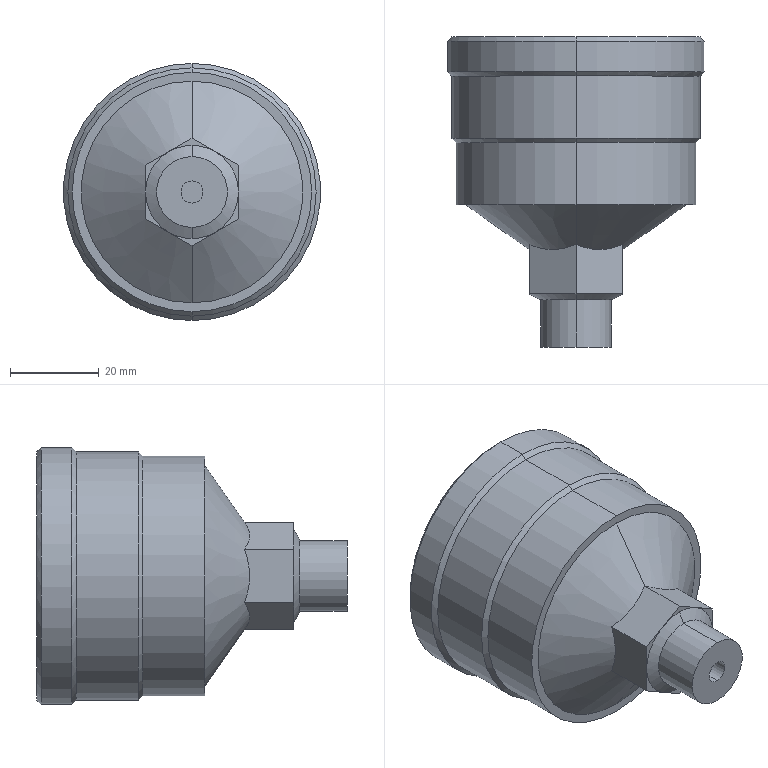Part | SolidWorks | features Boss 1, Revolution 1 | 1 solid | 41 faces | box 58 x 70 x 58 mm | volume 93422 mm3 | plane 17 | cylinder 12 | cone 12 | commonest cylinder face diameters 5 x2 16 x2 26.006 x2 54 x2 56 x2 58 x2
STEP:
#1=CARTESIAN_POINT('',(0.,0.,-2.5));
#2=VERTEX_POINT('',#1);
#3=CARTESIAN_POINT('',(0.,0.,2.5));
#4=VERTEX_POINT('',#3);
#5=CARTESIAN_POINT('',(0.,0.,0.));
#6=DIRECTION('',(0.,1.,0.));
#7=DIRECTION('',(0.,0.,1.));
#8=AXIS2_PLACEMENT_3D('',#5,#6,#7);
#9=CIRCLE('',#8,2.5);
#10=EDGE_CURVE('',#2,#4,#9,.T.);
#11=ORIENTED_EDGE('',*,*,#10,.F.);
#12=CARTESIAN_POINT('',(0.,12.,-2.5));
#13=VERTEX_POINT('',#12);
#14=CARTESIAN_POINT('',(0.,0.,-2.5));
#15=DIRECTION('',(0.,1.,0.));
#16=VECTOR('',#15,1000.);
#17=LINE('',#14,#16);
#18=EDGE_CURVE('',#2,#13,#17,.T.);
#19=ORIENTED_EDGE('',*,*,#18,.T.);
#20=CARTESIAN_POINT('',(0.,12.,2.5));
#21=VERTEX_POINT('',#20);
#22=CARTESIAN_POINT('',(0.,12.,0.));
#23=DIRECTION('',(0.,-1.,0.));
#24=DIRECTION('',(0.,0.,-1.));
#25=AXIS2_PLACEMENT_3D('',#22,#23,#24);
#26=CIRCLE('',#25,2.5);
#27=EDGE_CURVE('',#21,#13,#26,.T.);
#28=ORIENTED_EDGE('',*,*,#27,.F.);
#29=CARTESIAN_POINT('',(0.,0.,2.5));
#30=DIRECTION('',(0.,1.,0.));
#31=VECTOR('',#30,1000.);
#32=LINE('',#29,#31);
#33=EDGE_CURVE('',#4,#21,#32,.T.);
#34=ORIENTED_EDGE('',*,*,#33,.F.);
#35=EDGE_LOOP('',(#11,#19,#28,#34));
#36=FACE_OUTER_BOUND('',#35,.T.);
#37=CARTESIAN_POINT('',(0.,0.,0.));
#38=DIRECTION('',(0.,1.,0.));
#39=DIRECTION('',(0.,0.,1.));
#40=AXIS2_PLACEMENT_3D('',#37,#38,#39);
#41=CYLINDRICAL_SURFACE('',#40,2.5);
#42=ADVANCED_FACE('',(#36),#41,.F.);
#43=CARTESIAN_POINT('',(0.,10.699,8.));
#44=VERTEX_POINT('',#43);
#45=CARTESIAN_POINT('',(0.,10.699,-8.));
#46=VERTEX_POINT('',#45);
#47=CARTESIAN_POINT('',(0.,10.699,0.));
#48=DIRECTION('',(0.,1.,0.));
#49=DIRECTION('',(0.,0.,1.));
#50=AXIS2_PLACEMENT_3D('',#47,#48,#49);
#51=CIRCLE('',#50,8.);
#52=EDGE_CURVE('',#44,#46,#51,.T.);
#53=ORIENTED_EDGE('',*,*,#52,.T.);
#54=CARTESIAN_POINT('',(0.,12.,-10.5));
#55=VERTEX_POINT('',#54);
#56=CARTESIAN_POINT('',(0.,12.,-10.5));
#57=DIRECTION('',(0.,0.4617,-0.887));
#58=VECTOR('',#57,1000.);
#59=LINE('',#56,#58);
#60=EDGE_CURVE('',#46,#55,#59,.T.);
#61=ORIENTED_EDGE('',*,*,#60,.T.);
#62=CARTESIAN_POINT('',(5.25,12.,-9.093));
#63=VERTEX_POINT('',#62);
#64=CARTESIAN_POINT('',(0.,12.,0.));
#65=DIRECTION('',(0.,1.,0.));
#66=DIRECTION('',(0.,0.,1.));
#67=AXIS2_PLACEMENT_3D('',#64,#65,#66);
#68=CIRCLE('',#67,10.5);
#69=EDGE_CURVE('',#63,#55,#68,.T.);
#70=ORIENTED_EDGE('',*,*,#69,.F.);
#71=CARTESIAN_POINT('',(10.5,12.,0.));
#72=VERTEX_POINT('',#71);
#73=CARTESIAN_POINT('',(0.,12.,0.));
#74=DIRECTION('',(0.,1.,0.));
#75=DIRECTION('',(0.,0.,1.));
#76=AXIS2_PLACEMENT_3D('',#73,#74,#75);
#77=CIRCLE('',#76,10.5);
#78=EDGE_CURVE('',#72,#63,#77,.T.);
#79=ORIENTED_EDGE('',*,*,#78,.F.);
#80=CARTESIAN_POINT('',(5.25,12.,9.093));
#81=VERTEX_POINT('',#80);
#82=CARTESIAN_POINT('',(0.,12.,0.));
#83=DIRECTION('',(0.,1.,0.));
#84=DIRECTION('',(0.,0.,1.));
#85=AXIS2_PLACEMENT_3D('',#82,#83,#84);
#86=CIRCLE('',#85,10.5);
#87=EDGE_CURVE('',#81,#72,#86,.T.);
#88=ORIENTED_EDGE('',*,*,#87,.F.);
#89=CARTESIAN_POINT('',(0.,12.,10.5));
#90=VERTEX_POINT('',#89);
#91=CARTESIAN_POINT('',(0.,12.,0.));
#92=DIRECTION('',(0.,1.,0.));
#93=DIRECTION('',(0.,0.,1.));
#94=AXIS2_PLACEMENT_3D('',#91,#92,#93);
#95=CIRCLE('',#94,10.5);
#96=EDGE_CURVE('',#90,#81,#95,.T.);
#97=ORIENTED_EDGE('',*,*,#96,.F.);
#98=CARTESIAN_POINT('',(0.,12.,10.5));
#99=DIRECTION('',(0.,0.4617,0.887));
#100=VECTOR('',#99,1000.);
#101=LINE('',#98,#100);
#102=EDGE_CURVE('',#44,#90,#101,.T.);
#103=ORIENTED_EDGE('',*,*,#102,.F.);
#104=EDGE_LOOP('',(#53,#61,#70,#79,#88,#97,#103));
#105=FACE_OUTER_BOUND('',#104,.T.);
#106=CARTESIAN_POINT('',(0.,12.,0.));
#107=DIRECTION('',(0.,1.,0.));
#108=DIRECTION('',(0.,0.,1.));
#109=AXIS2_PLACEMENT_3D('',#106,#107,#108);
#110=CONICAL_SURFACE('',#109,10.5,1.091);
#111=ADVANCED_FACE('',(#105),#110,.T.);
#112=CARTESIAN_POINT('',(0.,0.,8.));
#113=VERTEX_POINT('',#112);
#114=CARTESIAN_POINT('',(0.,0.,-8.));
#115=VERTEX_POINT('',#114);
#116=CARTESIAN_POINT('',(0.,0.,0.));
#117=DIRECTION('',(0.,1.,0.));
#118=DIRECTION('',(0.,0.,1.));
#119=AXIS2_PLACEMENT_3D('',#116,#117,#118);
#120=CIRCLE('',#119,8.);
#121=EDGE_CURVE('',#113,#115,#120,.T.);
#122=ORIENTED_EDGE('',*,*,#121,.T.);
#123=CARTESIAN_POINT('',(0.,0.,-8.));
#124=DIRECTION('',(0.,1.,0.));
#125=VECTOR('',#124,1000.);
#126=LINE('',#123,#125);
#127=EDGE_CURVE('',#115,#46,#126,.T.);
#128=ORIENTED_EDGE('',*,*,#127,.T.);
#129=ORIENTED_EDGE('',*,*,#52,.F.);
#130=CARTESIAN_POINT('',(0.,0.,8.));
#131=DIRECTION('',(0.,1.,0.));
#132=VECTOR('',#131,1000.);
#133=LINE('',#130,#132);
#134=EDGE_CURVE('',#113,#44,#133,.T.);
#135=ORIENTED_EDGE('',*,*,#134,.F.);
#136=EDGE_LOOP('',(#122,#128,#129,#135));
#137=FACE_OUTER_BOUND('',#136,.T.);
#138=CARTESIAN_POINT('',(0.,0.,0.));
#139=DIRECTION('',(0.,1.,0.));
#140=DIRECTION('',(0.,0.,1.));
#141=AXIS2_PLACEMENT_3D('',#138,#139,#140);
#142=CYLINDRICAL_SURFACE('',#141,8.);
#143=ADVANCED_FACE('',(#137),#142,.T.);
#144=CARTESIAN_POINT('',(0.,70.,28.));
#145=VERTEX_POINT('',#144);
#146=CARTESIAN_POINT('',(0.,70.,-28.));
#147=VERTEX_POINT('',#146);
#148=CARTESIAN_POINT('',(0.,70.,0.));
#149=DIRECTION('',(0.,1.,0.));
#150=DIRECTION('',(0.,0.,1.));
#151=AXIS2_PLACEMENT_3D('',#148,#149,#150);
#152=CIRCLE('',#151,28.);
#153=EDGE_CURVE('',#145,#147,#152,.T.);
#154=ORIENTED_EDGE('',*,*,#153,.F.);
#155=CARTESIAN_POINT('',(0.,69.,29.));
#156=VERTEX_POINT('',#155);
#157=CARTESIAN_POINT('',(0.,70.,28.));
#158=DIRECTION('',(0.,-0.7071,0.7071));
#159=VECTOR('',#158,1000.);
#160=LINE('',#157,#159);
#161=EDGE_CURVE('',#145,#156,#160,.T.);
#162=ORIENTED_EDGE('',*,*,#161,.T.);
#163=CARTESIAN_POINT('',(0.,69.,-29.));
#164=VERTEX_POINT('',#163);
#165=CARTESIAN_POINT('',(0.,69.,0.));
#166=DIRECTION('',(0.,1.,0.));
#167=DIRECTION('',(0.,0.,1.));
#168=AXIS2_PLACEMENT_3D('',#165,#166,#167);
#169=CIRCLE('',#168,29.);
#170=EDGE_CURVE('',#156,#164,#169,.T.);
#171=ORIENTED_EDGE('',*,*,#170,.T.);
#172=CARTESIAN_POINT('',(0.,70.,-28.));
#173=DIRECTION('',(0.,-0.7071,-0.7071));
#174=VECTOR('',#173,1000.);
#175=LINE('',#172,#174);
#176=EDGE_CURVE('',#147,#164,#175,.T.);
#177=ORIENTED_EDGE('',*,*,#176,.F.);
#178=EDGE_LOOP('',(#154,#162,#171,#177));
#179=FACE_OUTER_BOUND('',#178,.T.);
#180=CARTESIAN_POINT('',(0.,70.,0.));
#181=DIRECTION('',(0.,-1.,0.));
#182=DIRECTION('',(0.,0.,-1.));
#183=AXIS2_PLACEMENT_3D('',#180,#181,#182);
#184=CONICAL_SURFACE('',#183,28.,0.7854);
#185=ADVANCED_FACE('',(#179),#184,.T.);
#186=CARTESIAN_POINT('',(0.,62.153,29.));
#187=VERTEX_POINT('',#186);
#188=CARTESIAN_POINT('',(0.,62.153,-29.));
#189=VERTEX_POINT('',#188);
#190=CARTESIAN_POINT('',(0.,62.153,0.));
#191=DIRECTION('',(0.,1.,0.));
#192=DIRECTION('',(0.,0.,1.));
#193=AXIS2_PLACEMENT_3D('',#190,#191,#192);
#194=CIRCLE('',#193,29.);
#195=EDGE_CURVE('',#187,#189,#194,.T.);
#196=ORIENTED_EDGE('',*,*,#195,.T.);
#197=CARTESIAN_POINT('',(0.,0.,-29.));
#198=DIRECTION('',(0.,1.,0.));
#199=VECTOR('',#198,1000.);
#200=LINE('',#197,#199);
#201=EDGE_CURVE('',#189,#164,#200,.T.);
#202=ORIENTED_EDGE('',*,*,#201,.T.);
#203=ORIENTED_EDGE('',*,*,#170,.F.);
#204=CARTESIAN_POINT('',(0.,0.,29.));
#205=DIRECTION('',(0.,1.,0.));
#206=VECTOR('',#205,1000.);
#207=LINE('',#204,#206);
#208=EDGE_CURVE('',#187,#156,#207,.T.);
#209=ORIENTED_EDGE('',*,*,#208,.F.);
#210=EDGE_LOOP('',(#196,#202,#203,#209));
#211=FACE_OUTER_BOUND('',#210,.T.);
#212=CARTESIAN_POINT('',(0.,0.,0.));
#213=DIRECTION('',(0.,1.,0.));
#214=DIRECTION('',(0.,0.,1.));
#215=AXIS2_PLACEMENT_3D('',#212,#213,#214);
#216=CYLINDRICAL_SURFACE('',#215,29.);
#217=ADVANCED_FACE('',(#211),#216,.T.);
#218=CARTESIAN_POINT('',(0.,61.153,28.));
#219=VERTEX_POINT('',#218);
#220=CARTESIAN_POINT('',(0.,61.153,-28.));
#221=VERTEX_POINT('',#220);
#222=CARTESIAN_POINT('',(0.,61.153,0.));
#223=DIRECTION('',(0.,1.,0.));
#224=DIRECTION('',(0.,0.,1.));
#225=AXIS2_PLACEMENT_3D('',#222,#223,#224);
#226=CIRCLE('',#225,28.);
#227=EDGE_CURVE('',#219,#221,#226,.T.);
#228=ORIENTED_EDGE('',*,*,#227,.T.);
#229=CARTESIAN_POINT('',(0.,62.153,-29.));
#230=DIRECTION('',(0.,0.7071,-0.7071));
#231=VECTOR('',#230,1000.);
#232=LINE('',#229,#231);
#233=EDGE_CURVE('',#221,#189,#232,.T.);
#234=ORIENTED_EDGE('',*,*,#233,.T.);
#235=ORIENTED_EDGE('',*,*,#195,.F.);
#236=CARTESIAN_POINT('',(0.,62.153,29.));
#237=DIRECTION('',(0.,0.7071,0.7071));
#238=VECTOR('',#237,1000.);
#239=LINE('',#236,#238);
#240=EDGE_CURVE('',#219,#187,#239,.T.);
#241=ORIENTED_EDGE('',*,*,#240,.F.);
#242=EDGE_LOOP('',(#228,#234,#235,#241));
#243=FACE_OUTER_BOUND('',#242,.T.);
#244=CARTESIAN_POINT('',(0.,62.153,0.));
#245=DIRECTION('',(0.,1.,0.));
#246=DIRECTION('',(0.,0.,1.));
#247=AXIS2_PLACEMENT_3D('',#244,#245,#246);
#248=CONICAL_SURFACE('',#247,29.,0.7854);
#249=ADVANCED_FACE('',(#243),#248,.T.);
#250=CARTESIAN_POINT('',(0.,47.153,28.));
#251=VERTEX_POINT('',#250);
#252=CARTESIAN_POINT('',(0.,47.153,-28.));
#253=VERTEX_POINT('',#252);
#254=CARTESIAN_POINT('',(0.,47.153,0.));
#255=DIRECTION('',(0.,1.,0.));
#256=DIRECTION('',(0.,0.,1.));
#257=AXIS2_PLACEMENT_3D('',#254,#255,#256);
#258=CIRCLE('',#257,28.);
#259=EDGE_CURVE('',#251,#253,#258,.T.);
#260=ORIENTED_EDGE('',*,*,#259,.T.);
#261=CARTESIAN_POINT('',(0.,0.,-28.));
#262=DIRECTION('',(0.,1.,0.));
#263=VECTOR('',#262,1000.);
#264=LINE('',#261,#263);
#265=EDGE_CURVE('',#253,#221,#264,.T.);
#266=ORIENTED_EDGE('',*,*,#265,.T.);
#267=ORIENTED_EDGE('',*,*,#227,.F.);
#268=CARTESIAN_POINT('',(0.,0.,28.));
#269=DIRECTION('',(0.,1.,0.));
#270=VECTOR('',#269,1000.);
#271=LINE('',#268,#270);
#272=EDGE_CURVE('',#251,#219,#271,.T.);
#273=ORIENTED_EDGE('',*,*,#272,.F.);
#274=EDGE_LOOP('',(#260,#266,#267,#273));
#275=FACE_OUTER_BOUND('',#274,.T.);
#276=CARTESIAN_POINT('',(0.,0.,0.));
#277=DIRECTION('',(0.,1.,0.));
#278=DIRECTION('',(0.,0.,1.));
#279=AXIS2_PLACEMENT_3D('',#276,#277,#278);
#280=CYLINDRICAL_SURFACE('',#279,28.);
#281=ADVANCED_FACE('',(#275),#280,.T.);
#282=CARTESIAN_POINT('',(0.,46.153,27.));
#283=VERTEX_POINT('',#282);
#284=CARTESIAN_POINT('',(0.,46.153,-27.));
#285=VERTEX_POINT('',#284);
#286=CARTESIAN_POINT('',(0.,46.153,0.));
#287=DIRECTION('',(0.,1.,0.));
#288=DIRECTION('',(0.,0.,1.));
#289=AXIS2_PLACEMENT_3D('',#286,#287,#288);
#290=CIRCLE('',#289,27.);
#291=EDGE_CURVE('',#283,#285,#290,.T.);
#292=ORIENTED_EDGE('',*,*,#291,.T.);
#293=CARTESIAN_POINT('',(0.,47.153,-28.));
#294=DIRECTION('',(0.,0.7071,-0.7071));
#295=VECTOR('',#294,1000.);
#296=LINE('',#293,#295);
#297=EDGE_CURVE('',#285,#253,#296,.T.);
#298=ORIENTED_EDGE('',*,*,#297,.T.);
#299=ORIENTED_EDGE('',*,*,#259,.F.);
#300=CARTESIAN_POINT('',(0.,47.153,28.));
#301=DIRECTION('',(0.,0.7071,0.7071));
#302=VECTOR('',#301,1000.);
#303=LINE('',#300,#302);
#304=EDGE_CURVE('',#283,#251,#303,.T.);
#305=ORIENTED_EDGE('',*,*,#304,.F.);
#306=EDGE_LOOP('',(#292,#298,#299,#305));
#307=FACE_OUTER_BOUND('',#306,.T.);
#308=CARTESIAN_POINT('',(0.,47.153,0.));
#309=DIRECTION('',(0.,1.,0.));
#310=DIRECTION('',(0.,0.,1.));
#311=AXIS2_PLACEMENT_3D('',#308,#309,#310);
#312=CONICAL_SURFACE('',#311,28.,0.7854);
#313=ADVANCED_FACE('',(#307),#312,.T.);
#314=CARTESIAN_POINT('',(0.,32.153,27.));
#315=VERTEX_POINT('',#314);
#316=CARTESIAN_POINT('',(0.,32.153,-27.));
#317=VERTEX_POINT('',#316);
#318=CARTESIAN_POINT('',(0.,32.153,0.));
#319=DIRECTION('',(0.,1.,0.));
#320=DIRECTION('',(0.,0.,1.));
#321=AXIS2_PLACEMENT_3D('',#318,#319,#320);
#322=CIRCLE('',#321,27.);
#323=EDGE_CURVE('',#315,#317,#322,.T.);
#324=ORIENTED_EDGE('',*,*,#323,.T.);
#325=CARTESIAN_POINT('',(0.,0.,-27.));
#326=DIRECTION('',(0.,1.,0.));
#327=VECTOR('',#326,1000.);
#328=LINE('',#325,#327);
#329=EDGE_CURVE('',#317,#285,#328,.T.);
#330=ORIENTED_EDGE('',*,*,#329,.T.);
#331=ORIENTED_EDGE('',*,*,#291,.F.);
#332=CARTESIAN_POINT('',(0.,0.,27.));
#333=DIRECTION('',(0.,1.,0.));
#334=VECTOR('',#333,1000.);
#335=LINE('',#332,#334);
#336=EDGE_CURVE('',#315,#283,#335,.T.);
#337=ORIENTED_EDGE('',*,*,#336,.F.);
#338=EDGE_LOOP('',(#324,#330,#331,#337));
#339=FACE_OUTER_BOUND('',#338,.T.);
#340=CARTESIAN_POINT('',(0.,0.,0.));
#341=DIRECTION('',(0.,1.,0.));
#342=DIRECTION('',(0.,0.,1.));
#343=AXIS2_PLACEMENT_3D('',#340,#341,#342);
#344=CYLINDRICAL_SURFACE('',#343,27.);
#345=ADVANCED_FACE('',(#339),#344,.T.);
#346=CARTESIAN_POINT('',(0.,32.153,-2.5));
#347=VERTEX_POINT('',#346);
#348=CARTESIAN_POINT('',(0.,32.153,2.5));
#349=VERTEX_POINT('',#348);
#350=CARTESIAN_POINT('',(0.,32.153,0.));
#351=DIRECTION('',(0.,1.,0.));
#352=DIRECTION('',(0.,0.,1.));
#353=AXIS2_PLACEMENT_3D('',#350,#351,#352);
#354=CIRCLE('',#353,2.5);
#355=EDGE_CURVE('',#347,#349,#354,.T.);
#356=ORIENTED_EDGE('',*,*,#355,.F.);
#357=CARTESIAN_POINT('',(0.,47.153,-13.003));
#358=VERTEX_POINT('',#357);
#359=CARTESIAN_POINT('',(0.,32.153,-2.5));
#360=DIRECTION('',(0.,0.8192,-0.5736));
#361=VECTOR('',#360,1000.);
#362=LINE('',#359,#361);
#363=EDGE_CURVE('',#347,#358,#362,.T.);
#364=ORIENTED_EDGE('',*,*,#363,.T.);
#365=CARTESIAN_POINT('',(0.,47.153,13.003));
#366=VERTEX_POINT('',#365);
#367=CARTESIAN_POINT('',(0.,47.153,0.));
#368=DIRECTION('',(0.,1.,0.));
#369=DIRECTION('',(0.,0.,1.));
#370=AXIS2_PLACEMENT_3D('',#367,#368,#369);
#371=CIRCLE('',#370,13.003);
#372=EDGE_CURVE('',#358,#366,#371,.T.);
#373=ORIENTED_EDGE('',*,*,#372,.T.);
#374=CARTESIAN_POINT('',(0.,32.153,2.5));
#375=DIRECTION('',(0.,0.8192,0.5736));
#376=VECTOR('',#375,1000.);
#377=LINE('',#374,#376);
#378=EDGE_CURVE('',#349,#366,#377,.T.);
#379=ORIENTED_EDGE('',*,*,#378,.F.);
#380=EDGE_LOOP('',(#356,#364,#373,#379));
#381=FACE_OUTER_BOUND('',#380,.T.);
#382=CARTESIAN_POINT('',(0.,32.153,0.));
#383=DIRECTION('',(0.,1.,0.));
#384=DIRECTION('',(0.,0.,1.));
#385=AXIS2_PLACEMENT_3D('',#382,#383,#384);
#386=CONICAL_SURFACE('',#385,2.5,0.6109);
#387=ADVANCED_FACE('',(#381),#386,.F.);
#388=ORIENTED_EDGE('',*,*,#372,.F.);
#389=CARTESIAN_POINT('',(0.,70.,-13.003));
#390=VERTEX_POINT('',#389);
#391=CARTESIAN_POINT('',(0.,0.,-13.003));
#392=DIRECTION('',(0.,1.,0.));
#393=VECTOR('',#392,1000.);
#394=LINE('',#391,#393);
#395=EDGE_CURVE('',#358,#390,#394,.T.);
#396=ORIENTED_EDGE('',*,*,#395,.T.);
#397=CARTESIAN_POINT('',(0.,70.,13.003));
#398=VERTEX_POINT('',#397);
#399=CARTESIAN_POINT('',(0.,70.,0.));
#400=DIRECTION('',(0.,1.,0.));
#401=DIRECTION('',(0.,0.,1.));
#402=AXIS2_PLACEMENT_3D('',#399,#400,#401);
#403=CIRCLE('',#402,13.003);
#404=EDGE_CURVE('',#390,#398,#403,.T.);
#405=ORIENTED_EDGE('',*,*,#404,.T.);
#406=CARTESIAN_POINT('',(0.,0.,13.003));
#407=DIRECTION('',(0.,1.,0.));
#408=VECTOR('',#407,1000.);
#409=LINE('',#406,#408);
#410=EDGE_CURVE('',#366,#398,#409,.T.);
#411=ORIENTED_EDGE('',*,*,#410,.F.);
#412=EDGE_LOOP('',(#388,#396,#405,#411));
#413=FACE_OUTER_BOUND('',#412,.T.);
#414=CARTESIAN_POINT('',(0.,0.,0.));
#415=DIRECTION('',(0.,1.,0.));
#416=DIRECTION('',(0.,0.,1.));
#417=AXIS2_PLACEMENT_3D('',#414,#415,#416);
#418=CYLINDRICAL_SURFACE('',#417,13.003);
#419=ADVANCED_FACE('',(#413),#418,.F.);
#420=CARTESIAN_POINT('',(10.5,23.137,-6.062));
#421=VERTEX_POINT('',#420);
#422=CARTESIAN_POINT('',(0.,23.137,-12.124));
#423=VERTEX_POINT('',#422);
#424=CARTESIAN_POINT('',(10.5,23.137,-6.062));
#425=CARTESIAN_POINT('',(9.651,22.794,-6.552));
#426=CARTESIAN_POINT('',(8.793,22.509,-7.048));
#427=CARTESIAN_POINT('',(7.053,22.113,-8.053));
#428=CARTESIAN_POINT('',(6.17,22.002,-8.562));
#429=CARTESIAN_POINT('',(4.821,21.999,-9.341));
#430=CARTESIAN_POINT('',(4.366,22.026,-9.603));
#431=CARTESIAN_POINT('',(3.472,22.131,-10.12));
#432=CARTESIAN_POINT('',(3.03,22.208,-10.375));
#433=CARTESIAN_POINT('',(1.713,22.507,-11.135));
#434=CARTESIAN_POINT('',(0.8515,22.793,-11.633));
#435=CARTESIAN_POINT('',(0.,23.137,-12.124));
#436=B_SPLINE_CURVE_WITH_KNOTS('',3,(#424,#425,#426,#427,#428,#429,#430,#431,#432,#433,#434,#435),.UNSPECIFIED.,.F.,.F.,(4,2,2,2,2,4),(0.000000241,0.003072,0.006144,0.00768,0.009216,0.01229),.UNSPECIFIED.);
#437=EDGE_CURVE('',#421,#423,#436,.T.);
#438=ORIENTED_EDGE('',*,*,#437,.T.);
#439=CARTESIAN_POINT('',(0.,32.153,-25.));
#440=VERTEX_POINT('',#439);
#441=CARTESIAN_POINT('',(0.,32.153,-25.));
#442=DIRECTION('',(0.,0.5736,-0.8192));
#443=VECTOR('',#442,1000.);
#444=LINE('',#441,#443);
#445=EDGE_CURVE('',#423,#440,#444,.T.);
#446=ORIENTED_EDGE('',*,*,#445,.T.);
#447=CARTESIAN_POINT('',(0.,32.153,25.));
#448=VERTEX_POINT('',#447);
#449=CARTESIAN_POINT('',(0.,32.153,0.));
#450=DIRECTION('',(0.,1.,0.));
#451=DIRECTION('',(0.,0.,1.));
#452=AXIS2_PLACEMENT_3D('',#449,#450,#451);
#453=CIRCLE('',#452,25.);
#454=EDGE_CURVE('',#448,#440,#453,.T.);
#455=ORIENTED_EDGE('',*,*,#454,.F.);
#456=CARTESIAN_POINT('',(0.,23.137,12.124));
#457=VERTEX_POINT('',#456);
#458=CARTESIAN_POINT('',(0.,32.153,25.));
#459=DIRECTION('',(0.,0.5736,0.8192));
#460=VECTOR('',#459,1000.);
#461=LINE('',#458,#460);
#462=EDGE_CURVE('',#457,#448,#461,.T.);
#463=ORIENTED_EDGE('',*,*,#462,.F.);
#464=CARTESIAN_POINT('',(10.5,23.137,6.062));
#465=VERTEX_POINT('',#464);
#466=CARTESIAN_POINT('',(0.,23.137,12.124));
#467=CARTESIAN_POINT('',(0.8491,22.794,11.634));
#468=CARTESIAN_POINT('',(1.707,22.509,11.139));
#469=CARTESIAN_POINT('',(3.447,22.113,10.134));
#470=CARTESIAN_POINT('',(4.33,22.002,9.624));
#471=CARTESIAN_POINT('',(5.679,21.999,8.846));
#472=CARTESIAN_POINT('',(6.134,22.026,8.583));
#473=CARTESIAN_POINT('',(7.028,22.131,8.067));
#474=CARTESIAN_POINT('',(7.47,22.208,7.811));
#475=CARTESIAN_POINT('',(8.787,22.507,7.051));
#476=CARTESIAN_POINT('',(9.648,22.793,6.554));
#477=CARTESIAN_POINT('',(10.5,23.137,6.062));
#478=B_SPLINE_CURVE_WITH_KNOTS('',3,(#466,#467,#468,#469,#470,#471,#472,#473,#474,#475,#476,#477),.UNSPECIFIED.,.F.,.F.,(4,2,2,2,2,4),(0.000000241,0.003072,0.006144,0.00768,0.009216,0.01229),.UNSPECIFIED.);
#479=EDGE_CURVE('',#457,#465,#478,.T.);
#480=ORIENTED_EDGE('',*,*,#479,.T.);
#481=CARTESIAN_POINT('',(10.5,23.137,6.062));
#482=CARTESIAN_POINT('',(10.5,22.797,5.089));
#483=CARTESIAN_POINT('',(10.5,22.511,4.1));
#484=CARTESIAN_POINT('',(10.5,22.211,2.58));
#485=CARTESIAN_POINT('',(10.5,22.133,2.068));
#486=CARTESIAN_POINT('',(10.5,22.026,1.029));
#487=CARTESIAN_POINT('',(10.5,22.,0.5092));
#488=CARTESIAN_POINT('',(10.5,22.,-1.038));
#489=CARTESIAN_POINT('',(10.5,22.109,-2.058));
#490=CARTESIAN_POINT('',(10.5,22.506,-4.08));
#491=CARTESIAN_POINT('',(10.5,22.796,-5.086));
#492=CARTESIAN_POINT('',(10.5,23.137,-6.062));
#493=B_SPLINE_CURVE_WITH_KNOTS('',3,(#481,#482,#483,#484,#485,#486,#487,#488,#489,#490,#491,#492),.UNSPECIFIED.,.F.,.F.,(4,2,2,2,2,4),(0.03191,0.03499,0.03653,0.03808,0.04116,0.04425),.UNSPECIFIED.);
#494=EDGE_CURVE('',#465,#421,#493,.T.);
#495=ORIENTED_EDGE('',*,*,#494,.T.);
#496=EDGE_LOOP('',(#438,#446,#455,#463,#480,#495));
#497=FACE_OUTER_BOUND('',#496,.T.);
#498=CARTESIAN_POINT('',(0.,32.153,0.));
#499=DIRECTION('',(0.,1.,0.));
#500=DIRECTION('',(0.,0.,1.));
#501=AXIS2_PLACEMENT_3D('',#498,#499,#500);
#502=CONICAL_SURFACE('',#501,25.,0.9599);
#503=ADVANCED_FACE('',(#497),#502,.T.);
#504=ORIENTED_EDGE('',*,*,#445,.F.);
#505=CARTESIAN_POINT('',(-10.5,23.137,-6.062));
#506=VERTEX_POINT('',#505);
#507=CARTESIAN_POINT('',(0.,23.137,-12.124));
#508=CARTESIAN_POINT('',(-0.8491,22.794,-11.634));
#509=CARTESIAN_POINT('',(-1.707,22.509,-11.139));
#510=CARTESIAN_POINT('',(-3.447,22.113,-10.134));
#511=CARTESIAN_POINT('',(-4.33,22.002,-9.624));
#512=CARTESIAN_POINT('',(-5.679,21.999,-8.846));
#513=CARTESIAN_POINT('',(-6.134,22.026,-8.583));
#514=CARTESIAN_POINT('',(-7.028,22.131,-8.067));
#515=CARTESIAN_POINT('',(-7.47,22.208,-7.811));
#516=CARTESIAN_POINT('',(-8.787,22.507,-7.051));
#517=CARTESIAN_POINT('',(-9.648,22.793,-6.554));
#518=CARTESIAN_POINT('',(-10.5,23.137,-6.062));
#519=B_SPLINE_CURVE_WITH_KNOTS('',3,(#507,#508,#509,#510,#511,#512,#513,#514,#515,#516,#517,#518),.UNSPECIFIED.,.F.,.F.,(4,2,2,2,2,4),(0.000000241,0.003072,0.006144,0.00768,0.009216,0.01229),.UNSPECIFIED.);
#520=EDGE_CURVE('',#423,#506,#519,.T.);
#521=ORIENTED_EDGE('',*,*,#520,.T.);
#522=CARTESIAN_POINT('',(-10.5,23.137,6.062));
#523=VERTEX_POINT('',#522);
#524=CARTESIAN_POINT('',(-10.5,23.137,-6.062));
#525=CARTESIAN_POINT('',(-10.5,22.796,-5.086));
#526=CARTESIAN_POINT('',(-10.5,22.506,-4.08));
#527=CARTESIAN_POINT('',(-10.5,22.109,-2.058));
#528=CARTESIAN_POINT('',(-10.5,22.,-1.038));
#529=CARTESIAN_POINT('',(-10.5,22.,0.5092));
#530=CARTESIAN_POINT('',(-10.5,22.026,1.029));
#531=CARTESIAN_POINT('',(-10.5,22.133,2.068));
#532=CARTESIAN_POINT('',(-10.5,22.211,2.58));
#533=CARTESIAN_POINT('',(-10.5,22.511,4.1));
#534=CARTESIAN_POINT('',(-10.5,22.797,5.089));
#535=CARTESIAN_POINT('',(-10.5,23.137,6.062));
#536=B_SPLINE_CURVE_WITH_KNOTS('',3,(#524,#525,#526,#527,#528,#529,#530,#531,#532,#533,#534,#535),.UNSPECIFIED.,.F.,.F.,(4,2,2,2,2,4),(0.01025,0.01333,0.01642,0.01796,0.01951,0.02259),.UNSPECIFIED.);
#537=EDGE_CURVE('',#506,#523,#536,.T.);
#538=ORIENTED_EDGE('',*,*,#537,.T.);
#539=CARTESIAN_POINT('',(-10.5,23.137,6.062));
#540=CARTESIAN_POINT('',(-9.651,22.794,6.552));
#541=CARTESIAN_POINT('',(-8.793,22.509,7.048));
#542=CARTESIAN_POINT('',(-7.053,22.113,8.053));
#543=CARTESIAN_POINT('',(-6.17,22.002,8.562));
#544=CARTESIAN_POINT('',(-4.821,21.999,9.341));
#545=CARTESIAN_POINT('',(-4.366,22.026,9.603));
#546=CARTESIAN_POINT('',(-3.472,22.131,10.12));
#547=CARTESIAN_POINT('',(-3.03,22.208,10.375));
#548=CARTESIAN_POINT('',(-1.713,22.507,11.135));
#549=CARTESIAN_POINT('',(-0.8515,22.793,11.633));
#550=CARTESIAN_POINT('',(0.,23.137,12.124));
#551=B_SPLINE_CURVE_WITH_KNOTS('',3,(#539,#540,#541,#542,#543,#544,#545,#546,#547,#548,#549,#550),.UNSPECIFIED.,.F.,.F.,(4,2,2,2,2,4),(0.000000241,0.003072,0.006144,0.00768,0.009216,0.01229),.UNSPECIFIED.);
#552=EDGE_CURVE('',#523,#457,#551,.T.);
#553=ORIENTED_EDGE('',*,*,#552,.T.);
#554=ORIENTED_EDGE('',*,*,#462,.T.);
#555=CARTESIAN_POINT('',(0.,32.153,0.));
#556=DIRECTION('',(0.,1.,0.));
#557=DIRECTION('',(0.,0.,1.));
#558=AXIS2_PLACEMENT_3D('',#555,#556,#557);
#559=CIRCLE('',#558,25.);
#560=EDGE_CURVE('',#440,#448,#559,.T.);
#561=ORIENTED_EDGE('',*,*,#560,.F.);
#562=EDGE_LOOP('',(#504,#521,#538,#553,#554,#561));
#563=FACE_OUTER_BOUND('',#562,.T.);
#564=CARTESIAN_POINT('',(0.,32.153,0.));
#565=DIRECTION('',(0.,1.,0.));
#566=DIRECTION('',(0.,0.,1.));
#567=AXIS2_PLACEMENT_3D('',#564,#565,#566);
#568=CONICAL_SURFACE('',#567,25.,0.9599);
#569=ADVANCED_FACE('',(#563),#568,.T.);
#570=CARTESIAN_POINT('',(0.,70.,0.));
#571=DIRECTION('',(0.,1.,0.));
#572=DIRECTION('',(0.,0.,1.));
#573=AXIS2_PLACEMENT_3D('',#570,#571,#572);
#574=CIRCLE('',#573,28.);
#575=EDGE_CURVE('',#147,#145,#574,.T.);
#576=ORIENTED_EDGE('',*,*,#575,.T.);
#577=ORIENTED_EDGE('',*,*,#153,.T.);
#578=EDGE_LOOP('',(#576,#577));
#579=FACE_OUTER_BOUND('',#578,.T.);
#580=CARTESIAN_POINT('',(0.,70.,0.));
#581=DIRECTION('',(0.,1.,0.));
#582=DIRECTION('',(0.,0.,1.));
#583=AXIS2_PLACEMENT_3D('',#580,#581,#582);
#584=CIRCLE('',#583,13.003);
#585=EDGE_CURVE('',#398,#390,#584,.T.);
#586=ORIENTED_EDGE('',*,*,#585,.F.);
#587=ORIENTED_EDGE('',*,*,#404,.F.);
#588=EDGE_LOOP('',(#586,#587));
#589=FACE_BOUND('',#588,.T.);
#590=CARTESIAN_POINT('',(-13.003,70.,0.));
#591=DIRECTION('',(0.,1.,0.));
#592=DIRECTION('',(0.,0.,1.));
#593=AXIS2_PLACEMENT_3D('',#590,#591,#592);
#594=PLANE('',#593);
#595=ADVANCED_FACE('',(#579,#589),#594,.T.);
#596=ORIENTED_EDGE('',*,*,#395,.F.);
#597=CARTESIAN_POINT('',(0.,47.153,0.));
#598=DIRECTION('',(0.,1.,0.));
#599=DIRECTION('',(0.,0.,1.));
#600=AXIS2_PLACEMENT_3D('',#597,#598,#599);
#601=CIRCLE('',#600,13.003);
#602=EDGE_CURVE('',#366,#358,#601,.T.);
#603=ORIENTED_EDGE('',*,*,#602,.F.);
#604=ORIENTED_EDGE('',*,*,#410,.T.);
#605=ORIENTED_EDGE('',*,*,#585,.T.);
#606=EDGE_LOOP('',(#596,#603,#604,#605));
#607=FACE_OUTER_BOUND('',#606,.T.);
#608=CARTESIAN_POINT('',(0.,0.,0.));
#609=DIRECTION('',(0.,1.,0.));
#610=DIRECTION('',(0.,0.,1.));
#611=AXIS2_PLACEMENT_3D('',#608,#609,#610);
#612=CYLINDRICAL_SURFACE('',#611,13.003);
#613=ADVANCED_FACE('',(#607),#612,.F.);
#614=ORIENTED_EDGE('',*,*,#363,.F.);
#615=CARTESIAN_POINT('',(0.,32.153,0.));
#616=DIRECTION('',(0.,1.,0.));
#617=DIRECTION('',(0.,0.,1.));
#618=AXIS2_PLACEMENT_3D('',#615,#616,#617);
#619=CIRCLE('',#618,2.5);
#620=EDGE_CURVE('',#349,#347,#619,.T.);
#621=ORIENTED_EDGE('',*,*,#620,.F.);
#622=ORIENTED_EDGE('',*,*,#378,.T.);
#623=ORIENTED_EDGE('',*,*,#602,.T.);
#624=EDGE_LOOP('',(#614,#621,#622,#623));
#625=FACE_OUTER_BOUND('',#624,.T.);
#626=CARTESIAN_POINT('',(0.,32.153,0.));
#627=DIRECTION('',(0.,1.,0.));
#628=DIRECTION('',(0.,0.,1.));
#629=AXIS2_PLACEMENT_3D('',#626,#627,#628);
#630=CONICAL_SURFACE('',#629,2.5,0.6109);
#631=ADVANCED_FACE('',(#625),#630,.F.);
#632=ORIENTED_EDGE('',*,*,#454,.T.);
#633=ORIENTED_EDGE('',*,*,#560,.T.);
#634=EDGE_LOOP('',(#632,#633));
#635=FACE_BOUND('',#634,.T.);
#636=ORIENTED_EDGE('',*,*,#323,.F.);
#637=CARTESIAN_POINT('',(0.,32.153,0.));
#638=DIRECTION('',(0.,1.,0.));
#639=DIRECTION('',(0.,0.,1.));
#640=AXIS2_PLACEMENT_3D('',#637,#638,#639);
#641=CIRCLE('',#640,27.);
#642=EDGE_CURVE('',#317,#315,#641,.T.);
#643=ORIENTED_EDGE('',*,*,#642,.F.);
#644=EDGE_LOOP('',(#636,#643));
#645=FACE_OUTER_BOUND('',#644,.T.);
#646=CARTESIAN_POINT('',(-27.,32.153,0.));
#647=DIRECTION('',(0.,-1.,0.));
#648=DIRECTION('',(0.,0.,-1.));
#649=AXIS2_PLACEMENT_3D('',#646,#647,#648);
#650=PLANE('',#649);
#651=ADVANCED_FACE('',(#635,#645),#650,.T.);
#652=ORIENTED_EDGE('',*,*,#329,.F.);
#653=ORIENTED_EDGE('',*,*,#642,.T.);
#654=ORIENTED_EDGE('',*,*,#336,.T.);
#655=CARTESIAN_POINT('',(0.,46.153,0.));
#656=DIRECTION('',(0.,1.,0.));
#657=DIRECTION('',(0.,0.,1.));
#658=AXIS2_PLACEMENT_3D('',#655,#656,#657);
#659=CIRCLE('',#658,27.);
#660=EDGE_CURVE('',#285,#283,#659,.T.);
#661=ORIENTED_EDGE('',*,*,#660,.F.);
#662=EDGE_LOOP('',(#652,#653,#654,#661));
#663=FACE_OUTER_BOUND('',#662,.T.);
#664=CARTESIAN_POINT('',(0.,0.,0.));
#665=DIRECTION('',(0.,1.,0.));
#666=DIRECTION('',(0.,0.,1.));
#667=AXIS2_PLACEMENT_3D('',#664,#665,#666);
#668=CYLINDRICAL_SURFACE('',#667,27.);
#669=ADVANCED_FACE('',(#663),#668,.T.);
#670=ORIENTED_EDGE('',*,*,#297,.F.);
#671=ORIENTED_EDGE('',*,*,#660,.T.);
#672=ORIENTED_EDGE('',*,*,#304,.T.);
#673=CARTESIAN_POINT('',(0.,47.153,0.));
#674=DIRECTION('',(0.,1.,0.));
#675=DIRECTION('',(0.,0.,1.));
#676=AXIS2_PLACEMENT_3D('',#673,#674,#675);
#677=CIRCLE('',#676,28.);
#678=EDGE_CURVE('',#253,#251,#677,.T.);
#679=ORIENTED_EDGE('',*,*,#678,.F.);
#680=EDGE_LOOP('',(#670,#671,#672,#679));
#681=FACE_OUTER_BOUND('',#680,.T.);
#682=CARTESIAN_POINT('',(0.,47.153,0.));
#683=DIRECTION('',(0.,1.,0.));
#684=DIRECTION('',(0.,0.,1.));
#685=AXIS2_PLACEMENT_3D('',#682,#683,#684);
#686=CONICAL_SURFACE('',#685,28.,0.7854);
#687=ADVANCED_FACE('',(#681),#686,.T.);
#688=ORIENTED_EDGE('',*,*,#265,.F.);
#689=ORIENTED_EDGE('',*,*,#678,.T.);
#690=ORIENTED_EDGE('',*,*,#272,.T.);
#691=CARTESIAN_POINT('',(0.,61.153,0.));
#692=DIRECTION('',(0.,1.,0.));
#693=DIRECTION('',(0.,0.,1.));
#694=AXIS2_PLACEMENT_3D('',#691,#692,#693);
#695=CIRCLE('',#694,28.);
#696=EDGE_CURVE('',#221,#219,#695,.T.);
#697=ORIENTED_EDGE('',*,*,#696,.F.);
#698=EDGE_LOOP('',(#688,#689,#690,#697));
#699=FACE_OUTER_BOUND('',#698,.T.);
#700=CARTESIAN_POINT('',(0.,0.,0.));
#701=DIRECTION('',(0.,1.,0.));
#702=DIRECTION('',(0.,0.,1.));
#703=AXIS2_PLACEMENT_3D('',#700,#701,#702);
#704=CYLINDRICAL_SURFACE('',#703,28.);
#705=ADVANCED_FACE('',(#699),#704,.T.);
#706=ORIENTED_EDGE('',*,*,#233,.F.);
#707=ORIENTED_EDGE('',*,*,#696,.T.);
#708=ORIENTED_EDGE('',*,*,#240,.T.);
#709=CARTESIAN_POINT('',(0.,62.153,0.));
#710=DIRECTION('',(0.,1.,0.));
#711=DIRECTION('',(0.,0.,1.));
#712=AXIS2_PLACEMENT_3D('',#709,#710,#711);
#713=CIRCLE('',#712,29.);
#714=EDGE_CURVE('',#189,#187,#713,.T.);
#715=ORIENTED_EDGE('',*,*,#714,.F.);
#716=EDGE_LOOP('',(#706,#707,#708,#715));
#717=FACE_OUTER_BOUND('',#716,.T.);
#718=CARTESIAN_POINT('',(0.,62.153,0.));
#719=DIRECTION('',(0.,1.,0.));
#720=DIRECTION('',(0.,0.,1.));
#721=AXIS2_PLACEMENT_3D('',#718,#719,#720);
#722=CONICAL_SURFACE('',#721,29.,0.7854);
#723=ADVANCED_FACE('',(#717),#722,.T.);
#724=ORIENTED_EDGE('',*,*,#201,.F.);
#725=ORIENTED_EDGE('',*,*,#714,.T.);
#726=ORIENTED_EDGE('',*,*,#208,.T.);
#727=CARTESIAN_POINT('',(0.,69.,0.));
#728=DIRECTION('',(0.,1.,0.));
#729=DIRECTION('',(0.,0.,1.));
#730=AXIS2_PLACEMENT_3D('',#727,#728,#729);
#731=CIRCLE('',#730,29.);
#732=EDGE_CURVE('',#164,#156,#731,.T.);
#733=ORIENTED_EDGE('',*,*,#732,.F.);
#734=EDGE_LOOP('',(#724,#725,#726,#733));
#735=FACE_OUTER_BOUND('',#734,.T.);
#736=CARTESIAN_POINT('',(0.,0.,0.));
#737=DIRECTION('',(0.,1.,0.));
#738=DIRECTION('',(0.,0.,1.));
#739=AXIS2_PLACEMENT_3D('',#736,#737,#738);
#740=CYLINDRICAL_SURFACE('',#739,29.);
#741=ADVANCED_FACE('',(#735),#740,.T.);
#742=ORIENTED_EDGE('',*,*,#161,.F.);
#743=ORIENTED_EDGE('',*,*,#575,.F.);
#744=ORIENTED_EDGE('',*,*,#176,.T.);
#745=ORIENTED_EDGE('',*,*,#732,.T.);
#746=EDGE_LOOP('',(#742,#743,#744,#745));
#747=FACE_OUTER_BOUND('',#746,.T.);
#748=CARTESIAN_POINT('',(0.,70.,0.));
#749=DIRECTION('',(0.,-1.,0.));
#750=DIRECTION('',(0.,0.,-1.));
#751=AXIS2_PLACEMENT_3D('',#748,#749,#750);
#752=CONICAL_SURFACE('',#751,28.,0.7854);
#753=ADVANCED_FACE('',(#747),#752,.T.);
#754=ORIENTED_EDGE('',*,*,#552,.F.);
#755=CARTESIAN_POINT('',(-10.5,12.,6.062));
#756=VERTEX_POINT('',#755);
#757=CARTESIAN_POINT('',(-10.5,32.153,6.062));
#758=DIRECTION('',(0.,-1.,0.));
#759=VECTOR('',#758,1000.);
#760=LINE('',#757,#759);
#761=EDGE_CURVE('',#523,#756,#760,.T.);
#762=ORIENTED_EDGE('',*,*,#761,.T.);
#763=CARTESIAN_POINT('',(-5.25,12.,9.093));
#764=VERTEX_POINT('',#763);
#765=CARTESIAN_POINT('',(-10.5,12.,6.062));
#766=DIRECTION('',(0.866,0.,0.5));
#767=VECTOR('',#766,1000.);
#768=LINE('',#765,#767);
#769=EDGE_CURVE('',#756,#764,#768,.T.);
#770=ORIENTED_EDGE('',*,*,#769,.T.);
#771=CARTESIAN_POINT('',(0.,12.,12.124));
#772=VERTEX_POINT('',#771);
#773=CARTESIAN_POINT('',(-10.5,12.,6.062));
#774=DIRECTION('',(0.866,0.,0.5));
#775=VECTOR('',#774,1000.);
#776=LINE('',#773,#775);
#777=EDGE_CURVE('',#764,#772,#776,.T.);
#778=ORIENTED_EDGE('',*,*,#777,.T.);
#779=CARTESIAN_POINT('',(0.,32.153,12.124));
#780=DIRECTION('',(0.,-1.,0.));
#781=VECTOR('',#780,1000.);
#782=LINE('',#779,#781);
#783=EDGE_CURVE('',#457,#772,#782,.T.);
#784=ORIENTED_EDGE('',*,*,#783,.F.);
#785=EDGE_LOOP('',(#754,#762,#770,#778,#784));
#786=FACE_OUTER_BOUND('',#785,.T.);
#787=CARTESIAN_POINT('',(-10.5,32.153,6.062));
#788=DIRECTION('',(0.5,0.,-0.866));
#789=DIRECTION('',(-0.866,0.,-0.5));
#790=AXIS2_PLACEMENT_3D('',#787,#788,#789);
#791=PLANE('',#790);
#792=ADVANCED_FACE('',(#786),#791,.F.);
#793=ORIENTED_EDGE('',*,*,#537,.F.);
#794=CARTESIAN_POINT('',(-10.5,12.,-6.062));
#795=VERTEX_POINT('',#794);
#796=CARTESIAN_POINT('',(-10.5,32.153,-6.062));
#797=DIRECTION('',(0.,-1.,0.));
#798=VECTOR('',#797,1000.);
#799=LINE('',#796,#798);
#800=EDGE_CURVE('',#506,#795,#799,.T.);
#801=ORIENTED_EDGE('',*,*,#800,.T.);
#802=CARTESIAN_POINT('',(-10.5,12.,0.));
#803=VERTEX_POINT('',#802);
#804=CARTESIAN_POINT('',(-10.5,12.,-6.062));
#805=DIRECTION('',(0.,0.,1.));
#806=VECTOR('',#805,1000.);
#807=LINE('',#804,#806);
#808=EDGE_CURVE('',#795,#803,#807,.T.);
#809=ORIENTED_EDGE('',*,*,#808,.T.);
#810=CARTESIAN_POINT('',(-10.5,12.,-6.062));
#811=DIRECTION('',(0.,0.,1.));
#812=VECTOR('',#811,1000.);
#813=LINE('',#810,#812);
#814=EDGE_CURVE('',#803,#756,#813,.T.);
#815=ORIENTED_EDGE('',*,*,#814,.T.);
#816=ORIENTED_EDGE('',*,*,#761,.F.);
#817=EDGE_LOOP('',(#793,#801,#809,#815,#816));
#818=FACE_OUTER_BOUND('',#817,.T.);
#819=CARTESIAN_POINT('',(-10.5,32.153,-6.062));
#820=DIRECTION('',(1.,0.,0.));
#821=DIRECTION('',(0.,0.,-1.));
#822=AXIS2_PLACEMENT_3D('',#819,#820,#821);
#823=PLANE('',#822);
#824=ADVANCED_FACE('',(#818),#823,.F.);
#825=ORIENTED_EDGE('',*,*,#520,.F.);
#826=CARTESIAN_POINT('',(0.,12.,-12.124));
#827=VERTEX_POINT('',#826);
#828=CARTESIAN_POINT('',(0.,32.153,-12.124));
#829=DIRECTION('',(0.,-1.,0.));
#830=VECTOR('',#829,1000.);
#831=LINE('',#828,#830);
#832=EDGE_CURVE('',#423,#827,#831,.T.);
#833=ORIENTED_EDGE('',*,*,#832,.T.);
#834=CARTESIAN_POINT('',(-5.25,12.,-9.093));
#835=VERTEX_POINT('',#834);
#836=CARTESIAN_POINT('',(0.,12.,-12.124));
#837=DIRECTION('',(-0.866,0.,0.5));
#838=VECTOR('',#837,1000.);
#839=LINE('',#836,#838);
#840=EDGE_CURVE('',#827,#835,#839,.T.);
#841=ORIENTED_EDGE('',*,*,#840,.T.);
#842=CARTESIAN_POINT('',(0.,12.,-12.124));
#843=DIRECTION('',(-0.866,0.,0.5));
#844=VECTOR('',#843,1000.);
#845=LINE('',#842,#844);
#846=EDGE_CURVE('',#835,#795,#845,.T.);
#847=ORIENTED_EDGE('',*,*,#846,.T.);
#848=ORIENTED_EDGE('',*,*,#800,.F.);
#849=EDGE_LOOP('',(#825,#833,#841,#847,#848));
#850=FACE_OUTER_BOUND('',#849,.T.);
#851=CARTESIAN_POINT('',(0.,32.153,-12.124));
#852=DIRECTION('',(0.5,0.,0.866));
#853=DIRECTION('',(0.866,0.,-0.5));
#854=AXIS2_PLACEMENT_3D('',#851,#852,#853);
#855=PLANE('',#854);
#856=ADVANCED_FACE('',(#850),#855,.F.);
#857=ORIENTED_EDGE('',*,*,#437,.F.);
#858=CARTESIAN_POINT('',(10.5,12.,-6.062));
#859=VERTEX_POINT('',#858);
#860=CARTESIAN_POINT('',(10.5,32.153,-6.062));
#861=DIRECTION('',(0.,-1.,0.));
#862=VECTOR('',#861,1000.);
#863=LINE('',#860,#862);
#864=EDGE_CURVE('',#421,#859,#863,.T.);
#865=ORIENTED_EDGE('',*,*,#864,.T.);
#866=CARTESIAN_POINT('',(10.5,12.,-6.062));
#867=DIRECTION('',(-0.866,0.,-0.5));
#868=VECTOR('',#867,1000.);
#869=LINE('',#866,#868);
#870=EDGE_CURVE('',#859,#63,#869,.T.);
#871=ORIENTED_EDGE('',*,*,#870,.T.);
#872=CARTESIAN_POINT('',(10.5,12.,-6.062));
#873=DIRECTION('',(-0.866,0.,-0.5));
#874=VECTOR('',#873,1000.);
#875=LINE('',#872,#874);
#876=EDGE_CURVE('',#63,#827,#875,.T.);
#877=ORIENTED_EDGE('',*,*,#876,.T.);
#878=ORIENTED_EDGE('',*,*,#832,.F.);
#879=EDGE_LOOP('',(#857,#865,#871,#877,#878));
#880=FACE_OUTER_BOUND('',#879,.T.);
#881=CARTESIAN_POINT('',(10.5,32.153,-6.062));
#882=DIRECTION('',(-0.5,0.,0.866));
#883=DIRECTION('',(0.866,0.,0.5));
#884=AXIS2_PLACEMENT_3D('',#881,#882,#883);
#885=PLANE('',#884);
#886=ADVANCED_FACE('',(#880),#885,.F.);
#887=ORIENTED_EDGE('',*,*,#494,.F.);
#888=CARTESIAN_POINT('',(10.5,12.,6.062));
#889=VERTEX_POINT('',#888);
#890=CARTESIAN_POINT('',(10.5,32.153,6.062));
#891=DIRECTION('',(0.,-1.,0.));
#892=VECTOR('',#891,1000.);
#893=LINE('',#890,#892);
#894=EDGE_CURVE('',#465,#889,#893,.T.);
#895=ORIENTED_EDGE('',*,*,#894,.T.);
#896=CARTESIAN_POINT('',(10.5,12.,6.062));
#897=DIRECTION('',(0.,0.,-1.));
#898=VECTOR('',#897,1000.);
#899=LINE('',#896,#898);
#900=EDGE_CURVE('',#889,#72,#899,.T.);
#901=ORIENTED_EDGE('',*,*,#900,.T.);
#902=CARTESIAN_POINT('',(10.5,12.,6.062));
#903=DIRECTION('',(0.,0.,-1.));
#904=VECTOR('',#903,1000.);
#905=LINE('',#902,#904);
#906=EDGE_CURVE('',#72,#859,#905,.T.);
#907=ORIENTED_EDGE('',*,*,#906,.T.);
#908=ORIENTED_EDGE('',*,*,#864,.F.);
#909=EDGE_LOOP('',(#887,#895,#901,#907,#908));
#910=FACE_OUTER_BOUND('',#909,.T.);
#911=CARTESIAN_POINT('',(10.5,32.153,6.062));
#912=DIRECTION('',(-1.,0.,0.));
#913=DIRECTION('',(0.,0.,1.));
#914=AXIS2_PLACEMENT_3D('',#911,#912,#913);
#915=PLANE('',#914);
#916=ADVANCED_FACE('',(#910),#915,.F.);
#917=ORIENTED_EDGE('',*,*,#479,.F.);
#918=ORIENTED_EDGE('',*,*,#783,.T.);
#919=CARTESIAN_POINT('',(0.,12.,12.124));
#920=DIRECTION('',(0.866,0.,-0.5));
#921=VECTOR('',#920,1000.);
#922=LINE('',#919,#921);
#923=EDGE_CURVE('',#772,#81,#922,.T.);
#924=ORIENTED_EDGE('',*,*,#923,.T.);
#925=CARTESIAN_POINT('',(0.,12.,12.124));
#926=DIRECTION('',(0.866,0.,-0.5));
#927=VECTOR('',#926,1000.);
#928=LINE('',#925,#927);
#929=EDGE_CURVE('',#81,#889,#928,.T.);
#930=ORIENTED_EDGE('',*,*,#929,.T.);
#931=ORIENTED_EDGE('',*,*,#894,.F.);
#932=EDGE_LOOP('',(#917,#918,#924,#930,#931));
#933=FACE_OUTER_BOUND('',#932,.T.);
#934=CARTESIAN_POINT('',(0.,32.153,12.124));
#935=DIRECTION('',(-0.5,0.,-0.866));
#936=DIRECTION('',(-0.866,0.,0.5));
#937=AXIS2_PLACEMENT_3D('',#934,#935,#936);
#938=PLANE('',#937);
#939=ADVANCED_FACE('',(#933),#938,.F.);
#940=ORIENTED_EDGE('',*,*,#876,.F.);
#941=ORIENTED_EDGE('',*,*,#69,.T.);
#942=CARTESIAN_POINT('',(0.,12.,0.));
#943=DIRECTION('',(0.,1.,0.));
#944=DIRECTION('',(0.,0.,1.));
#945=AXIS2_PLACEMENT_3D('',#942,#943,#944);
#946=CIRCLE('',#945,10.5);
#947=EDGE_CURVE('',#55,#835,#946,.T.);
#948=ORIENTED_EDGE('',*,*,#947,.T.);
#949=ORIENTED_EDGE('',*,*,#840,.F.);
#950=EDGE_LOOP('',(#940,#941,#948,#949));
#951=FACE_OUTER_BOUND('',#950,.T.);
#952=CARTESIAN_POINT('',(0.,12.,12.124));
#953=DIRECTION('',(0.,-1.,0.));
#954=DIRECTION('',(0.,0.,-1.));
#955=AXIS2_PLACEMENT_3D('',#952,#953,#954);
#956=PLANE('',#955);
#957=ADVANCED_FACE('',(#951),#956,.T.);
#958=ORIENTED_EDGE('',*,*,#906,.F.);
#959=ORIENTED_EDGE('',*,*,#78,.T.);
#960=ORIENTED_EDGE('',*,*,#870,.F.);
#961=EDGE_LOOP('',(#958,#959,#960));
#962=FACE_OUTER_BOUND('',#961,.T.);
#963=CARTESIAN_POINT('',(0.,12.,12.124));
#964=DIRECTION('',(0.,-1.,0.));
#965=DIRECTION('',(0.,0.,-1.));
#966=AXIS2_PLACEMENT_3D('',#963,#964,#965);
#967=PLANE('',#966);
#968=ADVANCED_FACE('',(#962),#967,.T.);
#969=ORIENTED_EDGE('',*,*,#929,.F.);
#970=ORIENTED_EDGE('',*,*,#87,.T.);
#971=ORIENTED_EDGE('',*,*,#900,.F.);
#972=EDGE_LOOP('',(#969,#970,#971));
#973=FACE_OUTER_BOUND('',#972,.T.);
#974=CARTESIAN_POINT('',(0.,12.,12.124));
#975=DIRECTION('',(0.,-1.,0.));
#976=DIRECTION('',(0.,0.,-1.));
#977=AXIS2_PLACEMENT_3D('',#974,#975,#976);
#978=PLANE('',#977);
#979=ADVANCED_FACE('',(#973),#978,.T.);
#980=ORIENTED_EDGE('',*,*,#777,.F.);
#981=CARTESIAN_POINT('',(0.,12.,0.));
#982=DIRECTION('',(0.,1.,0.));
#983=DIRECTION('',(0.,0.,1.));
#984=AXIS2_PLACEMENT_3D('',#981,#982,#983);
#985=CIRCLE('',#984,10.5);
#986=EDGE_CURVE('',#764,#90,#985,.T.);
#987=ORIENTED_EDGE('',*,*,#986,.T.);
#988=ORIENTED_EDGE('',*,*,#96,.T.);
#989=ORIENTED_EDGE('',*,*,#923,.F.);
#990=EDGE_LOOP('',(#980,#987,#988,#989));
#991=FACE_OUTER_BOUND('',#990,.T.);
#992=CARTESIAN_POINT('',(0.,12.,12.124));
#993=DIRECTION('',(0.,-1.,0.));
#994=DIRECTION('',(0.,0.,-1.));
#995=AXIS2_PLACEMENT_3D('',#992,#993,#994);
#996=PLANE('',#995);
#997=ADVANCED_FACE('',(#991),#996,.T.);
#998=ORIENTED_EDGE('',*,*,#814,.F.);
#999=CARTESIAN_POINT('',(0.,12.,0.));
#1000=DIRECTION('',(0.,1.,0.));
#1001=DIRECTION('',(0.,0.,1.));
#1002=AXIS2_PLACEMENT_3D('',#999,#1000,#1001);
#1003=CIRCLE('',#1002,10.5);
#1004=EDGE_CURVE('',#803,#764,#1003,.T.);
#1005=ORIENTED_EDGE('',*,*,#1004,.T.);
#1006=ORIENTED_EDGE('',*,*,#769,.F.);
#1007=EDGE_LOOP('',(#998,#1005,#1006));
#1008=FACE_OUTER_BOUND('',#1007,.T.);
#1009=CARTESIAN_POINT('',(0.,12.,12.124));
#1010=DIRECTION('',(0.,-1.,0.));
#1011=DIRECTION('',(0.,0.,-1.));
#1012=AXIS2_PLACEMENT_3D('',#1009,#1010,#1011);
#1013=PLANE('',#1012);
#1014=ADVANCED_FACE('',(#1008),#1013,.T.);
#1015=ORIENTED_EDGE('',*,*,#846,.F.);
#1016=CARTESIAN_POINT('',(0.,12.,0.));
#1017=DIRECTION('',(0.,1.,0.));
#1018=DIRECTION('',(0.,0.,1.));
#1019=AXIS2_PLACEMENT_3D('',#1016,#1017,#1018);
#1020=CIRCLE('',#1019,10.5);
#1021=EDGE_CURVE('',#835,#803,#1020,.T.);
#1022=ORIENTED_EDGE('',*,*,#1021,.T.);
#1023=ORIENTED_EDGE('',*,*,#808,.F.);
#1024=EDGE_LOOP('',(#1015,#1022,#1023));
#1025=FACE_OUTER_BOUND('',#1024,.T.);
#1026=CARTESIAN_POINT('',(0.,12.,12.124));
#1027=DIRECTION('',(0.,-1.,0.));
#1028=DIRECTION('',(0.,0.,-1.));
#1029=AXIS2_PLACEMENT_3D('',#1026,#1027,#1028);
#1030=PLANE('',#1029);
#1031=ADVANCED_FACE('',(#1025),#1030,.T.);
#1032=ORIENTED_EDGE('',*,*,#127,.F.);
#1033=CARTESIAN_POINT('',(0.,0.,0.));
#1034=DIRECTION('',(0.,1.,0.));
#1035=DIRECTION('',(0.,0.,1.));
#1036=AXIS2_PLACEMENT_3D('',#1033,#1034,#1035);
#1037=CIRCLE('',#1036,8.);
#1038=EDGE_CURVE('',#115,#113,#1037,.T.);
#1039=ORIENTED_EDGE('',*,*,#1038,.T.);
#1040=ORIENTED_EDGE('',*,*,#134,.T.);
#1041=CARTESIAN_POINT('',(0.,10.699,0.));
#1042=DIRECTION('',(0.,1.,0.));
#1043=DIRECTION('',(0.,0.,1.));
#1044=AXIS2_PLACEMENT_3D('',#1041,#1042,#1043);
#1045=CIRCLE('',#1044,8.);
#1046=EDGE_CURVE('',#46,#44,#1045,.T.);
#1047=ORIENTED_EDGE('',*,*,#1046,.F.);
#1048=EDGE_LOOP('',(#1032,#1039,#1040,#1047));
#1049=FACE_OUTER_BOUND('',#1048,.T.);
#1050=CARTESIAN_POINT('',(0.,0.,0.));
#1051=DIRECTION('',(0.,1.,0.));
#1052=DIRECTION('',(0.,0.,1.));
#1053=AXIS2_PLACEMENT_3D('',#1050,#1051,#1052);
#1054=CYLINDRICAL_SURFACE('',#1053,8.);
#1055=ADVANCED_FACE('',(#1049),#1054,.T.);
#1056=ORIENTED_EDGE('',*,*,#60,.F.);
#1057=ORIENTED_EDGE('',*,*,#1046,.T.);
#1058=ORIENTED_EDGE('',*,*,#102,.T.);
#1059=ORIENTED_EDGE('',*,*,#986,.F.);
#1060=ORIENTED_EDGE('',*,*,#1004,.F.);
#1061=ORIENTED_EDGE('',*,*,#1021,.F.);
#1062=ORIENTED_EDGE('',*,*,#947,.F.);
#1063=EDGE_LOOP('',(#1056,#1057,#1058,#1059,#1060,#1061,#1062));
#1064=FACE_OUTER_BOUND('',#1063,.T.);
#1065=CARTESIAN_POINT('',(0.,12.,0.));
#1066=DIRECTION('',(0.,1.,0.));
#1067=DIRECTION('',(0.,0.,1.));
#1068=AXIS2_PLACEMENT_3D('',#1065,#1066,#1067);
#1069=CONICAL_SURFACE('',#1068,10.5,1.091);
#1070=ADVANCED_FACE('',(#1064),#1069,.T.);
#1071=CARTESIAN_POINT('',(0.,0.,0.));
#1072=DIRECTION('',(0.,1.,0.));
#1073=DIRECTION('',(0.,0.,1.));
#1074=AXIS2_PLACEMENT_3D('',#1071,#1072,#1073);
#1075=CIRCLE('',#1074,2.5);
#1076=EDGE_CURVE('',#4,#2,#1075,.T.);
#1077=ORIENTED_EDGE('',*,*,#1076,.T.);
#1078=ORIENTED_EDGE('',*,*,#10,.T.);
#1079=EDGE_LOOP('',(#1077,#1078));
#1080=FACE_BOUND('',#1079,.T.);
#1081=ORIENTED_EDGE('',*,*,#121,.F.);
#1082=ORIENTED_EDGE('',*,*,#1038,.F.);
#1083=EDGE_LOOP('',(#1081,#1082));
#1084=FACE_OUTER_BOUND('',#1083,.T.);
#1085=CARTESIAN_POINT('',(-8.,0.,0.));
#1086=DIRECTION('',(0.,-1.,0.));
#1087=DIRECTION('',(0.,0.,-1.));
#1088=AXIS2_PLACEMENT_3D('',#1085,#1086,#1087);
#1089=PLANE('',#1088);
#1090=ADVANCED_FACE('',(#1080,#1084),#1089,.T.);
#1091=ORIENTED_EDGE('',*,*,#18,.F.);
#1092=ORIENTED_EDGE('',*,*,#1076,.F.);
#1093=ORIENTED_EDGE('',*,*,#33,.T.);
#1094=CARTESIAN_POINT('',(0.,12.,0.));
#1095=DIRECTION('',(0.,-1.,0.));
#1096=DIRECTION('',(0.,0.,-1.));
#1097=AXIS2_PLACEMENT_3D('',#1094,#1095,#1096);
#1098=CIRCLE('',#1097,2.5);
#1099=EDGE_CURVE('',#13,#21,#1098,.T.);
#1100=ORIENTED_EDGE('',*,*,#1099,.F.);
#1101=EDGE_LOOP('',(#1091,#1092,#1093,#1100));
#1102=FACE_OUTER_BOUND('',#1101,.T.);
#1103=CARTESIAN_POINT('',(0.,0.,0.));
#1104=DIRECTION('',(0.,1.,0.));
#1105=DIRECTION('',(0.,0.,1.));
#1106=AXIS2_PLACEMENT_3D('',#1103,#1104,#1105);
#1107=CYLINDRICAL_SURFACE('',#1106,2.5);
#1108=ADVANCED_FACE('',(#1102),#1107,.F.);
#1109=ORIENTED_EDGE('',*,*,#27,.T.);
#1110=ORIENTED_EDGE('',*,*,#1099,.T.);
#1111=EDGE_LOOP('',(#1109,#1110));
#1112=FACE_OUTER_BOUND('',#1111,.T.);
#1113=CARTESIAN_POINT('',(0.,12.,12.124));
#1114=DIRECTION('',(0.,-1.,0.));
#1115=DIRECTION('',(0.,0.,-1.));
#1116=AXIS2_PLACEMENT_3D('',#1113,#1114,#1115);
#1117=PLANE('',#1116);
#1118=ADVANCED_FACE('',(#1112),#1117,.T.);
#1119=ORIENTED_EDGE('',*,*,#620,.T.);
#1120=ORIENTED_EDGE('',*,*,#355,.T.);
#1121=EDGE_LOOP('',(#1119,#1120));
#1122=FACE_OUTER_BOUND('',#1121,.T.);
#1123=CARTESIAN_POINT('',(0.,32.153,12.124));
#1124=DIRECTION('',(0.,-1.,0.));
#1125=DIRECTION('',(0.,0.,-1.));
#1126=AXIS2_PLACEMENT_3D('',#1123,#1124,#1125);
#1127=PLANE('',#1126);
#1128=ADVANCED_FACE('',(#1122),#1127,.F.);
#1129=CLOSED_SHELL('',(#42,#111,#143,#185,#217,#249,#281,#313,#345,#387,#419,#503,#569,#595,#613,#631,#651,#669,#687,#705,#723,#741,#753,#792,#824,#856,#886,#916,#939,#957,#968,#979,#997,#1014,#1031,#1055,#1070,#1090,#1108,#1118,#1128));
#1130=MANIFOLD_SOLID_BREP('',#1129);
#1131=CARTESIAN_POINT('',(0.,0.,0.));
#1132=DIRECTION('',(0.,0.,1.));
#1133=DIRECTION('',(1.,0.,0.));
#1134=AXIS2_PLACEMENT_3D('',#1131,#1132,#1133);
#1135=(LENGTH_UNIT()NAMED_UNIT(*)SI_UNIT(.MILLI.,.METRE.));
#1136=UNCERTAINTY_MEASURE_WITH_UNIT(LENGTH_MEASURE(0.00001),#1135,'','');
#1137=(NAMED_UNIT(*)PLANE_ANGLE_UNIT()SI_UNIT($,.RADIAN.));
#1138=(NAMED_UNIT(*)SI_UNIT($,.STERADIAN.)SOLID_ANGLE_UNIT());
#1139=(GEOMETRIC_REPRESENTATION_CONTEXT(3)GLOBAL_UNCERTAINTY_ASSIGNED_CONTEXT((#1136))GLOBAL_UNIT_ASSIGNED_CONTEXT((#1135,#1137,#1138))REPRESENTATION_CONTEXT('',''));
#1140=ADVANCED_BREP_SHAPE_REPRESENTATION('',(#1130,#1134),#1139);